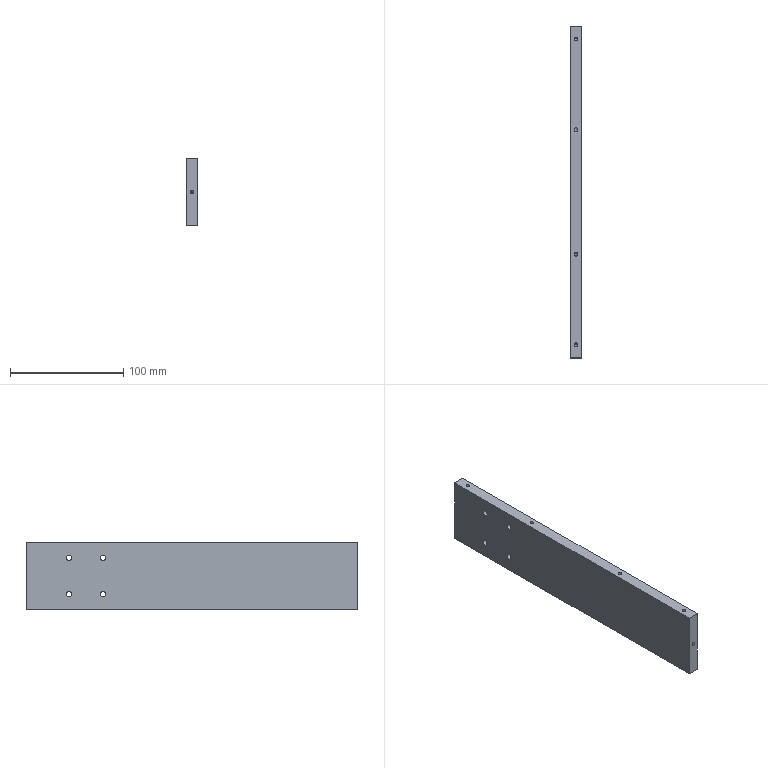Part | SolidWorks | features HoleWzd 3, MirrorPattern 2, Extrusion 1 | 1 solid | 54 faces | box 10 x 293 x 60 mm | volume 174003 mm3 | cylinder 28 | cone 20 | plane 6 | commonest cylinder face diameters 3.3 x20 5 x8
STEP:
#1=CARTESIAN_POINT('',(1.65,135.,-18.5));
#2=VERTEX_POINT('',#1);
#3=CARTESIAN_POINT('',(-1.65,135.,-18.5));
#4=VERTEX_POINT('',#3);
#5=CARTESIAN_POINT('',(0.,135.,-18.5));
#6=DIRECTION('',(0.,0.,-1.));
#7=DIRECTION('',(-1.,0.,0.));
#8=AXIS2_PLACEMENT_3D('',#5,#6,#7);
#9=CIRCLE('',#8,1.65);
#10=EDGE_CURVE('',#2,#4,#9,.T.);
#11=ORIENTED_EDGE('',*,*,#10,.F.);
#12=CARTESIAN_POINT('',(1.65,135.,-30.));
#13=VERTEX_POINT('',#12);
#14=CARTESIAN_POINT('',(1.65,135.,-30.));
#15=DIRECTION('',(0.,0.,-1.));
#16=VECTOR('',#15,1000.);
#17=LINE('',#14,#16);
#18=EDGE_CURVE('',#2,#13,#17,.T.);
#19=ORIENTED_EDGE('',*,*,#18,.T.);
#20=CARTESIAN_POINT('',(-1.65,135.,-30.));
#21=VERTEX_POINT('',#20);
#22=CARTESIAN_POINT('',(0.,135.,-30.));
#23=DIRECTION('',(0.,0.,-1.));
#24=DIRECTION('',(-1.,0.,0.));
#25=AXIS2_PLACEMENT_3D('',#22,#23,#24);
#26=CIRCLE('',#25,1.65);
#27=EDGE_CURVE('',#13,#21,#26,.T.);
#28=ORIENTED_EDGE('',*,*,#27,.T.);
#29=CARTESIAN_POINT('',(-1.65,135.,-30.));
#30=DIRECTION('',(0.,0.,-1.));
#31=VECTOR('',#30,1000.);
#32=LINE('',#29,#31);
#33=EDGE_CURVE('',#4,#21,#32,.T.);
#34=ORIENTED_EDGE('',*,*,#33,.F.);
#35=EDGE_LOOP('',(#11,#19,#28,#34));
#36=FACE_OUTER_BOUND('',#35,.T.);
#37=CARTESIAN_POINT('',(0.,135.,-30.));
#38=DIRECTION('',(0.,0.,-1.));
#39=DIRECTION('',(-1.,0.,0.));
#40=AXIS2_PLACEMENT_3D('',#37,#38,#39);
#41=CYLINDRICAL_SURFACE('',#40,1.65);
#42=ADVANCED_FACE('',(#36),#41,.F.);
#43=CARTESIAN_POINT('',(0.,135.,-17.509));
#44=VERTEX_POINT('',#43);
#45=CARTESIAN_POINT('',(-1.65,135.,-18.5));
#46=DIRECTION('',(-0.8572,0.,-0.515));
#47=VECTOR('',#46,1000.);
#48=LINE('',#45,#47);
#49=EDGE_CURVE('',#44,#4,#48,.T.);
#50=ORIENTED_EDGE('',*,*,#49,.F.);
#51=CARTESIAN_POINT('',(1.65,135.,-18.5));
#52=DIRECTION('',(0.8572,0.,-0.515));
#53=VECTOR('',#52,1000.);
#54=LINE('',#51,#53);
#55=EDGE_CURVE('',#44,#2,#54,.T.);
#56=ORIENTED_EDGE('',*,*,#55,.T.);
#57=ORIENTED_EDGE('',*,*,#10,.T.);
#58=EDGE_LOOP('',(#50,#56,#57));
#59=FACE_OUTER_BOUND('',#58,.T.);
#60=CARTESIAN_POINT('',(0.,135.,-18.5));
#61=DIRECTION('',(0.,0.,-1.));
#62=DIRECTION('',(-1.,0.,0.));
#63=AXIS2_PLACEMENT_3D('',#60,#61,#62);
#64=CONICAL_SURFACE('',#63,1.65,1.03);
#65=ADVANCED_FACE('',(#59),#64,.F.);
#66=CARTESIAN_POINT('',(1.65,-135.,-18.5));
#67=VERTEX_POINT('',#66);
#68=CARTESIAN_POINT('',(-1.65,-135.,-18.5));
#69=VERTEX_POINT('',#68);
#70=CARTESIAN_POINT('',(0.,-135.,-18.5));
#71=DIRECTION('',(0.,0.,-1.));
#72=DIRECTION('',(-1.,0.,0.));
#73=AXIS2_PLACEMENT_3D('',#70,#71,#72);
#74=CIRCLE('',#73,1.65);
#75=EDGE_CURVE('',#67,#69,#74,.T.);
#76=ORIENTED_EDGE('',*,*,#75,.F.);
#77=CARTESIAN_POINT('',(1.65,-135.,-30.));
#78=VERTEX_POINT('',#77);
#79=CARTESIAN_POINT('',(1.65,-135.,-30.));
#80=DIRECTION('',(0.,0.,-1.));
#81=VECTOR('',#80,1000.);
#82=LINE('',#79,#81);
#83=EDGE_CURVE('',#67,#78,#82,.T.);
#84=ORIENTED_EDGE('',*,*,#83,.T.);
#85=CARTESIAN_POINT('',(-1.65,-135.,-30.));
#86=VERTEX_POINT('',#85);
#87=CARTESIAN_POINT('',(0.,-135.,-30.));
#88=DIRECTION('',(0.,0.,-1.));
#89=DIRECTION('',(-1.,0.,0.));
#90=AXIS2_PLACEMENT_3D('',#87,#88,#89);
#91=CIRCLE('',#90,1.65);
#92=EDGE_CURVE('',#78,#86,#91,.T.);
#93=ORIENTED_EDGE('',*,*,#92,.T.);
#94=CARTESIAN_POINT('',(-1.65,-135.,-30.));
#95=DIRECTION('',(0.,0.,-1.));
#96=VECTOR('',#95,1000.);
#97=LINE('',#94,#96);
#98=EDGE_CURVE('',#69,#86,#97,.T.);
#99=ORIENTED_EDGE('',*,*,#98,.F.);
#100=EDGE_LOOP('',(#76,#84,#93,#99));
#101=FACE_OUTER_BOUND('',#100,.T.);
#102=CARTESIAN_POINT('',(0.,-135.,-30.));
#103=DIRECTION('',(0.,0.,-1.));
#104=DIRECTION('',(-1.,0.,0.));
#105=AXIS2_PLACEMENT_3D('',#102,#103,#104);
#106=CYLINDRICAL_SURFACE('',#105,1.65);
#107=ADVANCED_FACE('',(#101),#106,.F.);
#108=CARTESIAN_POINT('',(0.,-135.,-17.509));
#109=VERTEX_POINT('',#108);
#110=CARTESIAN_POINT('',(-1.65,-135.,-18.5));
#111=DIRECTION('',(-0.8572,0.,-0.515));
#112=VECTOR('',#111,1000.);
#113=LINE('',#110,#112);
#114=EDGE_CURVE('',#109,#69,#113,.T.);
#115=ORIENTED_EDGE('',*,*,#114,.F.);
#116=CARTESIAN_POINT('',(1.65,-135.,-18.5));
#117=DIRECTION('',(0.8572,0.,-0.515));
#118=VECTOR('',#117,1000.);
#119=LINE('',#116,#118);
#120=EDGE_CURVE('',#109,#67,#119,.T.);
#121=ORIENTED_EDGE('',*,*,#120,.T.);
#122=ORIENTED_EDGE('',*,*,#75,.T.);
#123=EDGE_LOOP('',(#115,#121,#122));
#124=FACE_OUTER_BOUND('',#123,.T.);
#125=CARTESIAN_POINT('',(0.,-135.,-18.5));
#126=DIRECTION('',(0.,0.,-1.));
#127=DIRECTION('',(-1.,0.,0.));
#128=AXIS2_PLACEMENT_3D('',#125,#126,#127);
#129=CONICAL_SURFACE('',#128,1.65,1.03);
#130=ADVANCED_FACE('',(#124),#129,.F.);
#131=CARTESIAN_POINT('',(1.65,55.,-18.5));
#132=VERTEX_POINT('',#131);
#133=CARTESIAN_POINT('',(-1.65,55.,-18.5));
#134=VERTEX_POINT('',#133);
#135=CARTESIAN_POINT('',(0.,55.,-18.5));
#136=DIRECTION('',(0.,0.,-1.));
#137=DIRECTION('',(-1.,0.,0.));
#138=AXIS2_PLACEMENT_3D('',#135,#136,#137);
#139=CIRCLE('',#138,1.65);
#140=EDGE_CURVE('',#132,#134,#139,.T.);
#141=ORIENTED_EDGE('',*,*,#140,.F.);
#142=CARTESIAN_POINT('',(1.65,55.,-30.));
#143=VERTEX_POINT('',#142);
#144=CARTESIAN_POINT('',(1.65,55.,-30.));
#145=DIRECTION('',(0.,0.,-1.));
#146=VECTOR('',#145,1000.);
#147=LINE('',#144,#146);
#148=EDGE_CURVE('',#132,#143,#147,.T.);
#149=ORIENTED_EDGE('',*,*,#148,.T.);
#150=CARTESIAN_POINT('',(-1.65,55.,-30.));
#151=VERTEX_POINT('',#150);
#152=CARTESIAN_POINT('',(0.,55.,-30.));
#153=DIRECTION('',(0.,0.,-1.));
#154=DIRECTION('',(-1.,0.,0.));
#155=AXIS2_PLACEMENT_3D('',#152,#153,#154);
#156=CIRCLE('',#155,1.65);
#157=EDGE_CURVE('',#143,#151,#156,.T.);
#158=ORIENTED_EDGE('',*,*,#157,.T.);
#159=CARTESIAN_POINT('',(-1.65,55.,-30.));
#160=DIRECTION('',(0.,0.,-1.));
#161=VECTOR('',#160,1000.);
#162=LINE('',#159,#161);
#163=EDGE_CURVE('',#134,#151,#162,.T.);
#164=ORIENTED_EDGE('',*,*,#163,.F.);
#165=EDGE_LOOP('',(#141,#149,#158,#164));
#166=FACE_OUTER_BOUND('',#165,.T.);
#167=CARTESIAN_POINT('',(0.,55.,-30.));
#168=DIRECTION('',(0.,0.,-1.));
#169=DIRECTION('',(-1.,0.,0.));
#170=AXIS2_PLACEMENT_3D('',#167,#168,#169);
#171=CYLINDRICAL_SURFACE('',#170,1.65);
#172=ADVANCED_FACE('',(#166),#171,.F.);
#173=CARTESIAN_POINT('',(0.,55.,-17.509));
#174=VERTEX_POINT('',#173);
#175=CARTESIAN_POINT('',(-1.65,55.,-18.5));
#176=DIRECTION('',(-0.8572,0.,-0.515));
#177=VECTOR('',#176,1000.);
#178=LINE('',#175,#177);
#179=EDGE_CURVE('',#174,#134,#178,.T.);
#180=ORIENTED_EDGE('',*,*,#179,.F.);
#181=CARTESIAN_POINT('',(1.65,55.,-18.5));
#182=DIRECTION('',(0.8572,0.,-0.515));
#183=VECTOR('',#182,1000.);
#184=LINE('',#181,#183);
#185=EDGE_CURVE('',#174,#132,#184,.T.);
#186=ORIENTED_EDGE('',*,*,#185,.T.);
#187=ORIENTED_EDGE('',*,*,#140,.T.);
#188=EDGE_LOOP('',(#180,#186,#187));
#189=FACE_OUTER_BOUND('',#188,.T.);
#190=CARTESIAN_POINT('',(0.,55.,-18.5));
#191=DIRECTION('',(0.,0.,-1.));
#192=DIRECTION('',(-1.,0.,0.));
#193=AXIS2_PLACEMENT_3D('',#190,#191,#192);
#194=CONICAL_SURFACE('',#193,1.65,1.03);
#195=ADVANCED_FACE('',(#189),#194,.F.);
#196=CARTESIAN_POINT('',(1.65,-55.,-18.5));
#197=VERTEX_POINT('',#196);
#198=CARTESIAN_POINT('',(-1.65,-55.,-18.5));
#199=VERTEX_POINT('',#198);
#200=CARTESIAN_POINT('',(0.,-55.,-18.5));
#201=DIRECTION('',(0.,0.,-1.));
#202=DIRECTION('',(-1.,0.,0.));
#203=AXIS2_PLACEMENT_3D('',#200,#201,#202);
#204=CIRCLE('',#203,1.65);
#205=EDGE_CURVE('',#197,#199,#204,.T.);
#206=ORIENTED_EDGE('',*,*,#205,.F.);
#207=CARTESIAN_POINT('',(1.65,-55.,-30.));
#208=VERTEX_POINT('',#207);
#209=CARTESIAN_POINT('',(1.65,-55.,-30.));
#210=DIRECTION('',(0.,0.,-1.));
#211=VECTOR('',#210,1000.);
#212=LINE('',#209,#211);
#213=EDGE_CURVE('',#197,#208,#212,.T.);
#214=ORIENTED_EDGE('',*,*,#213,.T.);
#215=CARTESIAN_POINT('',(-1.65,-55.,-30.));
#216=VERTEX_POINT('',#215);
#217=CARTESIAN_POINT('',(0.,-55.,-30.));
#218=DIRECTION('',(0.,0.,-1.));
#219=DIRECTION('',(-1.,0.,0.));
#220=AXIS2_PLACEMENT_3D('',#217,#218,#219);
#221=CIRCLE('',#220,1.65);
#222=EDGE_CURVE('',#208,#216,#221,.T.);
#223=ORIENTED_EDGE('',*,*,#222,.T.);
#224=CARTESIAN_POINT('',(-1.65,-55.,-30.));
#225=DIRECTION('',(0.,0.,-1.));
#226=VECTOR('',#225,1000.);
#227=LINE('',#224,#226);
#228=EDGE_CURVE('',#199,#216,#227,.T.);
#229=ORIENTED_EDGE('',*,*,#228,.F.);
#230=EDGE_LOOP('',(#206,#214,#223,#229));
#231=FACE_OUTER_BOUND('',#230,.T.);
#232=CARTESIAN_POINT('',(0.,-55.,-30.));
#233=DIRECTION('',(0.,0.,-1.));
#234=DIRECTION('',(-1.,0.,0.));
#235=AXIS2_PLACEMENT_3D('',#232,#233,#234);
#236=CYLINDRICAL_SURFACE('',#235,1.65);
#237=ADVANCED_FACE('',(#231),#236,.F.);
#238=CARTESIAN_POINT('',(0.,-55.,-17.509));
#239=VERTEX_POINT('',#238);
#240=CARTESIAN_POINT('',(-1.65,-55.,-18.5));
#241=DIRECTION('',(-0.8572,0.,-0.515));
#242=VECTOR('',#241,1000.);
#243=LINE('',#240,#242);
#244=EDGE_CURVE('',#239,#199,#243,.T.);
#245=ORIENTED_EDGE('',*,*,#244,.F.);
#246=CARTESIAN_POINT('',(1.65,-55.,-18.5));
#247=DIRECTION('',(0.8572,0.,-0.515));
#248=VECTOR('',#247,1000.);
#249=LINE('',#246,#248);
#250=EDGE_CURVE('',#239,#197,#249,.T.);
#251=ORIENTED_EDGE('',*,*,#250,.T.);
#252=ORIENTED_EDGE('',*,*,#205,.T.);
#253=EDGE_LOOP('',(#245,#251,#252));
#254=FACE_OUTER_BOUND('',#253,.T.);
#255=CARTESIAN_POINT('',(0.,-55.,-18.5));
#256=DIRECTION('',(0.,0.,-1.));
#257=DIRECTION('',(-1.,0.,0.));
#258=AXIS2_PLACEMENT_3D('',#255,#256,#257);
#259=CONICAL_SURFACE('',#258,1.65,1.03);
#260=ADVANCED_FACE('',(#254),#259,.F.);
#261=CARTESIAN_POINT('',(-5.,78.5,18.5));
#262=VERTEX_POINT('',#261);
#263=CARTESIAN_POINT('',(-5.,78.5,13.5));
#264=VERTEX_POINT('',#263);
#265=CARTESIAN_POINT('',(-5.,78.5,16.));
#266=DIRECTION('',(1.,0.,0.));
#267=DIRECTION('',(0.,0.,-1.));
#268=AXIS2_PLACEMENT_3D('',#265,#266,#267);
#269=CIRCLE('',#268,2.5);
#270=EDGE_CURVE('',#262,#264,#269,.T.);
#271=ORIENTED_EDGE('',*,*,#270,.F.);
#272=CARTESIAN_POINT('',(5.,78.5,18.5));
#273=VERTEX_POINT('',#272);
#274=CARTESIAN_POINT('',(5.,78.5,18.5));
#275=DIRECTION('',(1.,0.,0.));
#276=VECTOR('',#275,1000.);
#277=LINE('',#274,#276);
#278=EDGE_CURVE('',#262,#273,#277,.T.);
#279=ORIENTED_EDGE('',*,*,#278,.T.);
#280=CARTESIAN_POINT('',(5.,78.5,13.5));
#281=VERTEX_POINT('',#280);
#282=CARTESIAN_POINT('',(5.,78.5,16.));
#283=DIRECTION('',(1.,0.,0.));
#284=DIRECTION('',(0.,0.,-1.));
#285=AXIS2_PLACEMENT_3D('',#282,#283,#284);
#286=CIRCLE('',#285,2.5);
#287=EDGE_CURVE('',#273,#281,#286,.T.);
#288=ORIENTED_EDGE('',*,*,#287,.T.);
#289=CARTESIAN_POINT('',(5.,78.5,13.5));
#290=DIRECTION('',(1.,0.,0.));
#291=VECTOR('',#290,1000.);
#292=LINE('',#289,#291);
#293=EDGE_CURVE('',#264,#281,#292,.T.);
#294=ORIENTED_EDGE('',*,*,#293,.F.);
#295=EDGE_LOOP('',(#271,#279,#288,#294));
#296=FACE_OUTER_BOUND('',#295,.T.);
#297=CARTESIAN_POINT('',(5.,78.5,16.));
#298=DIRECTION('',(1.,0.,0.));
#299=DIRECTION('',(0.,0.,-1.));
#300=AXIS2_PLACEMENT_3D('',#297,#298,#299);
#301=CYLINDRICAL_SURFACE('',#300,2.5);
#302=ADVANCED_FACE('',(#296),#301,.F.);
#303=CARTESIAN_POINT('',(-5.,78.5,-13.5));
#304=VERTEX_POINT('',#303);
#305=CARTESIAN_POINT('',(-5.,78.5,-18.5));
#306=VERTEX_POINT('',#305);
#307=CARTESIAN_POINT('',(-5.,78.5,-16.));
#308=DIRECTION('',(1.,0.,0.));
#309=DIRECTION('',(0.,0.,-1.));
#310=AXIS2_PLACEMENT_3D('',#307,#308,#309);
#311=CIRCLE('',#310,2.5);
#312=EDGE_CURVE('',#304,#306,#311,.T.);
#313=ORIENTED_EDGE('',*,*,#312,.F.);
#314=CARTESIAN_POINT('',(5.,78.5,-13.5));
#315=VERTEX_POINT('',#314);
#316=CARTESIAN_POINT('',(5.,78.5,-13.5));
#317=DIRECTION('',(1.,0.,0.));
#318=VECTOR('',#317,1000.);
#319=LINE('',#316,#318);
#320=EDGE_CURVE('',#304,#315,#319,.T.);
#321=ORIENTED_EDGE('',*,*,#320,.T.);
#322=CARTESIAN_POINT('',(5.,78.5,-18.5));
#323=VERTEX_POINT('',#322);
#324=CARTESIAN_POINT('',(5.,78.5,-16.));
#325=DIRECTION('',(1.,0.,0.));
#326=DIRECTION('',(0.,0.,-1.));
#327=AXIS2_PLACEMENT_3D('',#324,#325,#326);
#328=CIRCLE('',#327,2.5);
#329=EDGE_CURVE('',#315,#323,#328,.T.);
#330=ORIENTED_EDGE('',*,*,#329,.T.);
#331=CARTESIAN_POINT('',(5.,78.5,-18.5));
#332=DIRECTION('',(1.,0.,0.));
#333=VECTOR('',#332,1000.);
#334=LINE('',#331,#333);
#335=EDGE_CURVE('',#306,#323,#334,.T.);
#336=ORIENTED_EDGE('',*,*,#335,.F.);
#337=EDGE_LOOP('',(#313,#321,#330,#336));
#338=FACE_OUTER_BOUND('',#337,.T.);
#339=CARTESIAN_POINT('',(5.,78.5,-16.));
#340=DIRECTION('',(1.,0.,0.));
#341=DIRECTION('',(0.,0.,-1.));
#342=AXIS2_PLACEMENT_3D('',#339,#340,#341);
#343=CYLINDRICAL_SURFACE('',#342,2.5);
#344=ADVANCED_FACE('',(#338),#343,.F.);
#345=CARTESIAN_POINT('',(-5.,108.5,-13.5));
#346=VERTEX_POINT('',#345);
#347=CARTESIAN_POINT('',(-5.,108.5,-18.5));
#348=VERTEX_POINT('',#347);
#349=CARTESIAN_POINT('',(-5.,108.5,-16.));
#350=DIRECTION('',(1.,0.,0.));
#351=DIRECTION('',(0.,0.,-1.));
#352=AXIS2_PLACEMENT_3D('',#349,#350,#351);
#353=CIRCLE('',#352,2.5);
#354=EDGE_CURVE('',#346,#348,#353,.T.);
#355=ORIENTED_EDGE('',*,*,#354,.F.);
#356=CARTESIAN_POINT('',(5.,108.5,-13.5));
#357=VERTEX_POINT('',#356);
#358=CARTESIAN_POINT('',(5.,108.5,-13.5));
#359=DIRECTION('',(1.,0.,0.));
#360=VECTOR('',#359,1000.);
#361=LINE('',#358,#360);
#362=EDGE_CURVE('',#346,#357,#361,.T.);
#363=ORIENTED_EDGE('',*,*,#362,.T.);
#364=CARTESIAN_POINT('',(5.,108.5,-18.5));
#365=VERTEX_POINT('',#364);
#366=CARTESIAN_POINT('',(5.,108.5,-16.));
#367=DIRECTION('',(1.,0.,0.));
#368=DIRECTION('',(0.,0.,-1.));
#369=AXIS2_PLACEMENT_3D('',#366,#367,#368);
#370=CIRCLE('',#369,2.5);
#371=EDGE_CURVE('',#357,#365,#370,.T.);
#372=ORIENTED_EDGE('',*,*,#371,.T.);
#373=CARTESIAN_POINT('',(5.,108.5,-18.5));
#374=DIRECTION('',(1.,0.,0.));
#375=VECTOR('',#374,1000.);
#376=LINE('',#373,#375);
#377=EDGE_CURVE('',#348,#365,#376,.T.);
#378=ORIENTED_EDGE('',*,*,#377,.F.);
#379=EDGE_LOOP('',(#355,#363,#372,#378));
#380=FACE_OUTER_BOUND('',#379,.T.);
#381=CARTESIAN_POINT('',(5.,108.5,-16.));
#382=DIRECTION('',(1.,0.,0.));
#383=DIRECTION('',(0.,0.,-1.));
#384=AXIS2_PLACEMENT_3D('',#381,#382,#383);
#385=CYLINDRICAL_SURFACE('',#384,2.5);
#386=ADVANCED_FACE('',(#380),#385,.F.);
#387=CARTESIAN_POINT('',(-5.,108.5,18.5));
#388=VERTEX_POINT('',#387);
#389=CARTESIAN_POINT('',(-5.,108.5,13.5));
#390=VERTEX_POINT('',#389);
#391=CARTESIAN_POINT('',(-5.,108.5,16.));
#392=DIRECTION('',(1.,0.,0.));
#393=DIRECTION('',(0.,0.,-1.));
#394=AXIS2_PLACEMENT_3D('',#391,#392,#393);
#395=CIRCLE('',#394,2.5);
#396=EDGE_CURVE('',#388,#390,#395,.T.);
#397=ORIENTED_EDGE('',*,*,#396,.F.);
#398=CARTESIAN_POINT('',(5.,108.5,18.5));
#399=VERTEX_POINT('',#398);
#400=CARTESIAN_POINT('',(5.,108.5,18.5));
#401=DIRECTION('',(1.,0.,0.));
#402=VECTOR('',#401,1000.);
#403=LINE('',#400,#402);
#404=EDGE_CURVE('',#388,#399,#403,.T.);
#405=ORIENTED_EDGE('',*,*,#404,.T.);
#406=CARTESIAN_POINT('',(5.,108.5,13.5));
#407=VERTEX_POINT('',#406);
#408=CARTESIAN_POINT('',(5.,108.5,16.));
#409=DIRECTION('',(1.,0.,0.));
#410=DIRECTION('',(0.,0.,-1.));
#411=AXIS2_PLACEMENT_3D('',#408,#409,#410);
#412=CIRCLE('',#411,2.5);
#413=EDGE_CURVE('',#399,#407,#412,.T.);
#414=ORIENTED_EDGE('',*,*,#413,.T.);
#415=CARTESIAN_POINT('',(5.,108.5,13.5));
#416=DIRECTION('',(1.,0.,0.));
#417=VECTOR('',#416,1000.);
#418=LINE('',#415,#417);
#419=EDGE_CURVE('',#390,#407,#418,.T.);
#420=ORIENTED_EDGE('',*,*,#419,.F.);
#421=EDGE_LOOP('',(#397,#405,#414,#420));
#422=FACE_OUTER_BOUND('',#421,.T.);
#423=CARTESIAN_POINT('',(5.,108.5,16.));
#424=DIRECTION('',(1.,0.,0.));
#425=DIRECTION('',(0.,0.,-1.));
#426=AXIS2_PLACEMENT_3D('',#423,#424,#425);
#427=CYLINDRICAL_SURFACE('',#426,2.5);
#428=ADVANCED_FACE('',(#422),#427,.F.);
#429=CARTESIAN_POINT('',(0.,135.,-1.65));
#430=VERTEX_POINT('',#429);
#431=CARTESIAN_POINT('',(0.,135.,1.65));
#432=VERTEX_POINT('',#431);
#433=CARTESIAN_POINT('',(0.,135.,0.));
#434=DIRECTION('',(0.,1.,0.));
#435=DIRECTION('',(0.,0.,1.));
#436=AXIS2_PLACEMENT_3D('',#433,#434,#435);
#437=CIRCLE('',#436,1.65);
#438=EDGE_CURVE('',#430,#432,#437,.T.);
#439=ORIENTED_EDGE('',*,*,#438,.F.);
#440=CARTESIAN_POINT('',(0.,146.5,-1.65));
#441=VERTEX_POINT('',#440);
#442=CARTESIAN_POINT('',(0.,146.5,-1.65));
#443=DIRECTION('',(0.,1.,0.));
#444=VECTOR('',#443,1000.);
#445=LINE('',#442,#444);
#446=EDGE_CURVE('',#430,#441,#445,.T.);
#447=ORIENTED_EDGE('',*,*,#446,.T.);
#448=CARTESIAN_POINT('',(0.,146.5,1.65));
#449=VERTEX_POINT('',#448);
#450=CARTESIAN_POINT('',(0.,146.5,0.));
#451=DIRECTION('',(0.,1.,0.));
#452=DIRECTION('',(0.,0.,1.));
#453=AXIS2_PLACEMENT_3D('',#450,#451,#452);
#454=CIRCLE('',#453,1.65);
#455=EDGE_CURVE('',#441,#449,#454,.T.);
#456=ORIENTED_EDGE('',*,*,#455,.T.);
#457=CARTESIAN_POINT('',(0.,146.5,1.65));
#458=DIRECTION('',(0.,1.,0.));
#459=VECTOR('',#458,1000.);
#460=LINE('',#457,#459);
#461=EDGE_CURVE('',#432,#449,#460,.T.);
#462=ORIENTED_EDGE('',*,*,#461,.F.);
#463=EDGE_LOOP('',(#439,#447,#456,#462));
#464=FACE_OUTER_BOUND('',#463,.T.);
#465=CARTESIAN_POINT('',(0.,146.5,0.));
#466=DIRECTION('',(0.,1.,0.));
#467=DIRECTION('',(0.,0.,1.));
#468=AXIS2_PLACEMENT_3D('',#465,#466,#467);
#469=CYLINDRICAL_SURFACE('',#468,1.65);
#470=ADVANCED_FACE('',(#464),#469,.F.);
#471=CARTESIAN_POINT('',(0.,134.009,0.));
#472=VERTEX_POINT('',#471);
#473=CARTESIAN_POINT('',(0.,135.,1.65));
#474=DIRECTION('',(0.,0.515,0.8572));
#475=VECTOR('',#474,1000.);
#476=LINE('',#473,#475);
#477=EDGE_CURVE('',#472,#432,#476,.T.);
#478=ORIENTED_EDGE('',*,*,#477,.F.);
#479=CARTESIAN_POINT('',(0.,135.,-1.65));
#480=DIRECTION('',(0.,0.515,-0.8572));
#481=VECTOR('',#480,1000.);
#482=LINE('',#479,#481);
#483=EDGE_CURVE('',#472,#430,#482,.T.);
#484=ORIENTED_EDGE('',*,*,#483,.T.);
#485=ORIENTED_EDGE('',*,*,#438,.T.);
#486=EDGE_LOOP('',(#478,#484,#485));
#487=FACE_OUTER_BOUND('',#486,.T.);
#488=CARTESIAN_POINT('',(0.,135.,0.));
#489=DIRECTION('',(0.,1.,0.));
#490=DIRECTION('',(0.,0.,1.));
#491=AXIS2_PLACEMENT_3D('',#488,#489,#490);
#492=CONICAL_SURFACE('',#491,1.65,1.03);
#493=ADVANCED_FACE('',(#487),#492,.F.);
#494=CARTESIAN_POINT('',(0.,-135.,1.65));
#495=VERTEX_POINT('',#494);
#496=CARTESIAN_POINT('',(0.,-135.,-1.65));
#497=VERTEX_POINT('',#496);
#498=CARTESIAN_POINT('',(0.,-135.,0.));
#499=DIRECTION('',(0.,-1.,0.));
#500=DIRECTION('',(0.,0.,-1.));
#501=AXIS2_PLACEMENT_3D('',#498,#499,#500);
#502=CIRCLE('',#501,1.65);
#503=EDGE_CURVE('',#495,#497,#502,.T.);
#504=ORIENTED_EDGE('',*,*,#503,.F.);
#505=CARTESIAN_POINT('',(0.,-146.5,1.65));
#506=VERTEX_POINT('',#505);
#507=CARTESIAN_POINT('',(0.,-146.5,1.65));
#508=DIRECTION('',(0.,-1.,0.));
#509=VECTOR('',#508,1000.);
#510=LINE('',#507,#509);
#511=EDGE_CURVE('',#495,#506,#510,.T.);
#512=ORIENTED_EDGE('',*,*,#511,.T.);
#513=CARTESIAN_POINT('',(0.,-146.5,-1.65));
#514=VERTEX_POINT('',#513);
#515=CARTESIAN_POINT('',(0.,-146.5,0.));
#516=DIRECTION('',(0.,-1.,0.));
#517=DIRECTION('',(0.,0.,-1.));
#518=AXIS2_PLACEMENT_3D('',#515,#516,#517);
#519=CIRCLE('',#518,1.65);
#520=EDGE_CURVE('',#506,#514,#519,.T.);
#521=ORIENTED_EDGE('',*,*,#520,.T.);
#522=CARTESIAN_POINT('',(0.,-146.5,-1.65));
#523=DIRECTION('',(0.,-1.,0.));
#524=VECTOR('',#523,1000.);
#525=LINE('',#522,#524);
#526=EDGE_CURVE('',#497,#514,#525,.T.);
#527=ORIENTED_EDGE('',*,*,#526,.F.);
#528=EDGE_LOOP('',(#504,#512,#521,#527));
#529=FACE_OUTER_BOUND('',#528,.T.);
#530=CARTESIAN_POINT('',(0.,-146.5,0.));
#531=DIRECTION('',(0.,-1.,0.));
#532=DIRECTION('',(0.,0.,-1.));
#533=AXIS2_PLACEMENT_3D('',#530,#531,#532);
#534=CYLINDRICAL_SURFACE('',#533,1.65);
#535=ADVANCED_FACE('',(#529),#534,.F.);
#536=CARTESIAN_POINT('',(0.,-134.009,0.));
#537=VERTEX_POINT('',#536);
#538=CARTESIAN_POINT('',(0.,-135.,-1.65));
#539=DIRECTION('',(0.,-0.515,-0.8572));
#540=VECTOR('',#539,1000.);
#541=LINE('',#538,#540);
#542=EDGE_CURVE('',#537,#497,#541,.T.);
#543=ORIENTED_EDGE('',*,*,#542,.F.);
#544=CARTESIAN_POINT('',(0.,-135.,1.65));
#545=DIRECTION('',(0.,-0.515,0.8572));
#546=VECTOR('',#545,1000.);
#547=LINE('',#544,#546);
#548=EDGE_CURVE('',#537,#495,#547,.T.);
#549=ORIENTED_EDGE('',*,*,#548,.T.);
#550=ORIENTED_EDGE('',*,*,#503,.T.);
#551=EDGE_LOOP('',(#543,#549,#550));
#552=FACE_OUTER_BOUND('',#551,.T.);
#553=CARTESIAN_POINT('',(0.,-135.,0.));
#554=DIRECTION('',(0.,-1.,0.));
#555=DIRECTION('',(0.,0.,-1.));
#556=AXIS2_PLACEMENT_3D('',#553,#554,#555);
#557=CONICAL_SURFACE('',#556,1.65,1.03);
#558=ADVANCED_FACE('',(#552),#557,.F.);
#559=CARTESIAN_POINT('',(-1.65,135.,18.5));
#560=VERTEX_POINT('',#559);
#561=CARTESIAN_POINT('',(1.65,135.,18.5));
#562=VERTEX_POINT('',#561);
#563=CARTESIAN_POINT('',(0.,135.,18.5));
#564=DIRECTION('',(0.,0.,1.));
#565=DIRECTION('',(1.,0.,0.));
#566=AXIS2_PLACEMENT_3D('',#563,#564,#565);
#567=CIRCLE('',#566,1.65);
#568=EDGE_CURVE('',#560,#562,#567,.T.);
#569=ORIENTED_EDGE('',*,*,#568,.F.);
#570=CARTESIAN_POINT('',(-1.65,135.,30.));
#571=VERTEX_POINT('',#570);
#572=CARTESIAN_POINT('',(-1.65,135.,30.));
#573=DIRECTION('',(0.,0.,1.));
#574=VECTOR('',#573,1000.);
#575=LINE('',#572,#574);
#576=EDGE_CURVE('',#560,#571,#575,.T.);
#577=ORIENTED_EDGE('',*,*,#576,.T.);
#578=CARTESIAN_POINT('',(1.65,135.,30.));
#579=VERTEX_POINT('',#578);
#580=CARTESIAN_POINT('',(0.,135.,30.));
#581=DIRECTION('',(0.,0.,1.));
#582=DIRECTION('',(1.,0.,0.));
#583=AXIS2_PLACEMENT_3D('',#580,#581,#582);
#584=CIRCLE('',#583,1.65);
#585=EDGE_CURVE('',#571,#579,#584,.T.);
#586=ORIENTED_EDGE('',*,*,#585,.T.);
#587=CARTESIAN_POINT('',(1.65,135.,30.));
#588=DIRECTION('',(0.,0.,1.));
#589=VECTOR('',#588,1000.);
#590=LINE('',#587,#589);
#591=EDGE_CURVE('',#562,#579,#590,.T.);
#592=ORIENTED_EDGE('',*,*,#591,.F.);
#593=EDGE_LOOP('',(#569,#577,#586,#592));
#594=FACE_OUTER_BOUND('',#593,.T.);
#595=CARTESIAN_POINT('',(0.,135.,30.));
#596=DIRECTION('',(0.,0.,1.));
#597=DIRECTION('',(1.,0.,0.));
#598=AXIS2_PLACEMENT_3D('',#595,#596,#597);
#599=CYLINDRICAL_SURFACE('',#598,1.65);
#600=ADVANCED_FACE('',(#594),#599,.F.);
#601=CARTESIAN_POINT('',(0.,135.,17.509));
#602=VERTEX_POINT('',#601);
#603=CARTESIAN_POINT('',(1.65,135.,18.5));
#604=DIRECTION('',(0.8572,0.,0.515));
#605=VECTOR('',#604,1000.);
#606=LINE('',#603,#605);
#607=EDGE_CURVE('',#602,#562,#606,.T.);
#608=ORIENTED_EDGE('',*,*,#607,.F.);
#609=CARTESIAN_POINT('',(-1.65,135.,18.5));
#610=DIRECTION('',(-0.8572,0.,0.515));
#611=VECTOR('',#610,1000.);
#612=LINE('',#609,#611);
#613=EDGE_CURVE('',#602,#560,#612,.T.);
#614=ORIENTED_EDGE('',*,*,#613,.T.);
#615=ORIENTED_EDGE('',*,*,#568,.T.);
#616=EDGE_LOOP('',(#608,#614,#615));
#617=FACE_OUTER_BOUND('',#616,.T.);
#618=CARTESIAN_POINT('',(0.,135.,18.5));
#619=DIRECTION('',(0.,0.,1.));
#620=DIRECTION('',(1.,0.,0.));
#621=AXIS2_PLACEMENT_3D('',#618,#619,#620);
#622=CONICAL_SURFACE('',#621,1.65,1.03);
#623=ADVANCED_FACE('',(#617),#622,.F.);
#624=CARTESIAN_POINT('',(-1.65,-135.,18.5));
#625=VERTEX_POINT('',#624);
#626=CARTESIAN_POINT('',(1.65,-135.,18.5));
#627=VERTEX_POINT('',#626);
#628=CARTESIAN_POINT('',(0.,-135.,18.5));
#629=DIRECTION('',(0.,0.,1.));
#630=DIRECTION('',(1.,0.,0.));
#631=AXIS2_PLACEMENT_3D('',#628,#629,#630);
#632=CIRCLE('',#631,1.65);
#633=EDGE_CURVE('',#625,#627,#632,.T.);
#634=ORIENTED_EDGE('',*,*,#633,.F.);
#635=CARTESIAN_POINT('',(-1.65,-135.,30.));
#636=VERTEX_POINT('',#635);
#637=CARTESIAN_POINT('',(-1.65,-135.,30.));
#638=DIRECTION('',(0.,0.,1.));
#639=VECTOR('',#638,1000.);
#640=LINE('',#637,#639);
#641=EDGE_CURVE('',#625,#636,#640,.T.);
#642=ORIENTED_EDGE('',*,*,#641,.T.);
#643=CARTESIAN_POINT('',(1.65,-135.,30.));
#644=VERTEX_POINT('',#643);
#645=CARTESIAN_POINT('',(0.,-135.,30.));
#646=DIRECTION('',(0.,0.,1.));
#647=DIRECTION('',(1.,0.,0.));
#648=AXIS2_PLACEMENT_3D('',#645,#646,#647);
#649=CIRCLE('',#648,1.65);
#650=EDGE_CURVE('',#636,#644,#649,.T.);
#651=ORIENTED_EDGE('',*,*,#650,.T.);
#652=CARTESIAN_POINT('',(1.65,-135.,30.));
#653=DIRECTION('',(0.,0.,1.));
#654=VECTOR('',#653,1000.);
#655=LINE('',#652,#654);
#656=EDGE_CURVE('',#627,#644,#655,.T.);
#657=ORIENTED_EDGE('',*,*,#656,.F.);
#658=EDGE_LOOP('',(#634,#642,#651,#657));
#659=FACE_OUTER_BOUND('',#658,.T.);
#660=CARTESIAN_POINT('',(0.,-135.,30.));
#661=DIRECTION('',(0.,0.,1.));
#662=DIRECTION('',(1.,0.,0.));
#663=AXIS2_PLACEMENT_3D('',#660,#661,#662);
#664=CYLINDRICAL_SURFACE('',#663,1.65);
#665=ADVANCED_FACE('',(#659),#664,.F.);
#666=CARTESIAN_POINT('',(0.,-135.,17.509));
#667=VERTEX_POINT('',#666);
#668=CARTESIAN_POINT('',(1.65,-135.,18.5));
#669=DIRECTION('',(0.8572,0.,0.515));
#670=VECTOR('',#669,1000.);
#671=LINE('',#668,#670);
#672=EDGE_CURVE('',#667,#627,#671,.T.);
#673=ORIENTED_EDGE('',*,*,#672,.F.);
#674=CARTESIAN_POINT('',(-1.65,-135.,18.5));
#675=DIRECTION('',(-0.8572,0.,0.515));
#676=VECTOR('',#675,1000.);
#677=LINE('',#674,#676);
#678=EDGE_CURVE('',#667,#625,#677,.T.);
#679=ORIENTED_EDGE('',*,*,#678,.T.);
#680=ORIENTED_EDGE('',*,*,#633,.T.);
#681=EDGE_LOOP('',(#673,#679,#680));
#682=FACE_OUTER_BOUND('',#681,.T.);
#683=CARTESIAN_POINT('',(0.,-135.,18.5));
#684=DIRECTION('',(0.,0.,1.));
#685=DIRECTION('',(1.,0.,0.));
#686=AXIS2_PLACEMENT_3D('',#683,#684,#685);
#687=CONICAL_SURFACE('',#686,1.65,1.03);
#688=ADVANCED_FACE('',(#682),#687,.F.);
#689=CARTESIAN_POINT('',(-1.65,55.,18.5));
#690=VERTEX_POINT('',#689);
#691=CARTESIAN_POINT('',(1.65,55.,18.5));
#692=VERTEX_POINT('',#691);
#693=CARTESIAN_POINT('',(0.,55.,18.5));
#694=DIRECTION('',(0.,0.,1.));
#695=DIRECTION('',(1.,0.,0.));
#696=AXIS2_PLACEMENT_3D('',#693,#694,#695);
#697=CIRCLE('',#696,1.65);
#698=EDGE_CURVE('',#690,#692,#697,.T.);
#699=ORIENTED_EDGE('',*,*,#698,.F.);
#700=CARTESIAN_POINT('',(-1.65,55.,30.));
#701=VERTEX_POINT('',#700);
#702=CARTESIAN_POINT('',(-1.65,55.,30.));
#703=DIRECTION('',(0.,0.,1.));
#704=VECTOR('',#703,1000.);
#705=LINE('',#702,#704);
#706=EDGE_CURVE('',#690,#701,#705,.T.);
#707=ORIENTED_EDGE('',*,*,#706,.T.);
#708=CARTESIAN_POINT('',(1.65,55.,30.));
#709=VERTEX_POINT('',#708);
#710=CARTESIAN_POINT('',(0.,55.,30.));
#711=DIRECTION('',(0.,0.,1.));
#712=DIRECTION('',(1.,0.,0.));
#713=AXIS2_PLACEMENT_3D('',#710,#711,#712);
#714=CIRCLE('',#713,1.65);
#715=EDGE_CURVE('',#701,#709,#714,.T.);
#716=ORIENTED_EDGE('',*,*,#715,.T.);
#717=CARTESIAN_POINT('',(1.65,55.,30.));
#718=DIRECTION('',(0.,0.,1.));
#719=VECTOR('',#718,1000.);
#720=LINE('',#717,#719);
#721=EDGE_CURVE('',#692,#709,#720,.T.);
#722=ORIENTED_EDGE('',*,*,#721,.F.);
#723=EDGE_LOOP('',(#699,#707,#716,#722));
#724=FACE_OUTER_BOUND('',#723,.T.);
#725=CARTESIAN_POINT('',(0.,55.,30.));
#726=DIRECTION('',(0.,0.,1.));
#727=DIRECTION('',(1.,0.,0.));
#728=AXIS2_PLACEMENT_3D('',#725,#726,#727);
#729=CYLINDRICAL_SURFACE('',#728,1.65);
#730=ADVANCED_FACE('',(#724),#729,.F.);
#731=CARTESIAN_POINT('',(0.,55.,17.509));
#732=VERTEX_POINT('',#731);
#733=CARTESIAN_POINT('',(1.65,55.,18.5));
#734=DIRECTION('',(0.8572,0.,0.515));
#735=VECTOR('',#734,1000.);
#736=LINE('',#733,#735);
#737=EDGE_CURVE('',#732,#692,#736,.T.);
#738=ORIENTED_EDGE('',*,*,#737,.F.);
#739=CARTESIAN_POINT('',(-1.65,55.,18.5));
#740=DIRECTION('',(-0.8572,0.,0.515));
#741=VECTOR('',#740,1000.);
#742=LINE('',#739,#741);
#743=EDGE_CURVE('',#732,#690,#742,.T.);
#744=ORIENTED_EDGE('',*,*,#743,.T.);
#745=ORIENTED_EDGE('',*,*,#698,.T.);
#746=EDGE_LOOP('',(#738,#744,#745));
#747=FACE_OUTER_BOUND('',#746,.T.);
#748=CARTESIAN_POINT('',(0.,55.,18.5));
#749=DIRECTION('',(0.,0.,1.));
#750=DIRECTION('',(1.,0.,0.));
#751=AXIS2_PLACEMENT_3D('',#748,#749,#750);
#752=CONICAL_SURFACE('',#751,1.65,1.03);
#753=ADVANCED_FACE('',(#747),#752,.F.);
#754=CARTESIAN_POINT('',(-1.65,-55.,18.5));
#755=VERTEX_POINT('',#754);
#756=CARTESIAN_POINT('',(1.65,-55.,18.5));
#757=VERTEX_POINT('',#756);
#758=CARTESIAN_POINT('',(0.,-55.,18.5));
#759=DIRECTION('',(0.,0.,1.));
#760=DIRECTION('',(1.,0.,0.));
#761=AXIS2_PLACEMENT_3D('',#758,#759,#760);
#762=CIRCLE('',#761,1.65);
#763=EDGE_CURVE('',#755,#757,#762,.T.);
#764=ORIENTED_EDGE('',*,*,#763,.F.);
#765=CARTESIAN_POINT('',(-1.65,-55.,30.));
#766=VERTEX_POINT('',#765);
#767=CARTESIAN_POINT('',(-1.65,-55.,30.));
#768=DIRECTION('',(0.,0.,1.));
#769=VECTOR('',#768,1000.);
#770=LINE('',#767,#769);
#771=EDGE_CURVE('',#755,#766,#770,.T.);
#772=ORIENTED_EDGE('',*,*,#771,.T.);
#773=CARTESIAN_POINT('',(1.65,-55.,30.));
#774=VERTEX_POINT('',#773);
#775=CARTESIAN_POINT('',(0.,-55.,30.));
#776=DIRECTION('',(0.,0.,1.));
#777=DIRECTION('',(1.,0.,0.));
#778=AXIS2_PLACEMENT_3D('',#775,#776,#777);
#779=CIRCLE('',#778,1.65);
#780=EDGE_CURVE('',#766,#774,#779,.T.);
#781=ORIENTED_EDGE('',*,*,#780,.T.);
#782=CARTESIAN_POINT('',(1.65,-55.,30.));
#783=DIRECTION('',(0.,0.,1.));
#784=VECTOR('',#783,1000.);
#785=LINE('',#782,#784);
#786=EDGE_CURVE('',#757,#774,#785,.T.);
#787=ORIENTED_EDGE('',*,*,#786,.F.);
#788=EDGE_LOOP('',(#764,#772,#781,#787));
#789=FACE_OUTER_BOUND('',#788,.T.);
#790=CARTESIAN_POINT('',(0.,-55.,30.));
#791=DIRECTION('',(0.,0.,1.));
#792=DIRECTION('',(1.,0.,0.));
#793=AXIS2_PLACEMENT_3D('',#790,#791,#792);
#794=CYLINDRICAL_SURFACE('',#793,1.65);
#795=ADVANCED_FACE('',(#789),#794,.F.);
#796=CARTESIAN_POINT('',(0.,-55.,17.509));
#797=VERTEX_POINT('',#796);
#798=CARTESIAN_POINT('',(1.65,-55.,18.5));
#799=DIRECTION('',(0.8572,0.,0.515));
#800=VECTOR('',#799,1000.);
#801=LINE('',#798,#800);
#802=EDGE_CURVE('',#797,#757,#801,.T.);
#803=ORIENTED_EDGE('',*,*,#802,.F.);
#804=CARTESIAN_POINT('',(-1.65,-55.,18.5));
#805=DIRECTION('',(-0.8572,0.,0.515));
#806=VECTOR('',#805,1000.);
#807=LINE('',#804,#806);
#808=EDGE_CURVE('',#797,#755,#807,.T.);
#809=ORIENTED_EDGE('',*,*,#808,.T.);
#810=ORIENTED_EDGE('',*,*,#763,.T.);
#811=EDGE_LOOP('',(#803,#809,#810));
#812=FACE_OUTER_BOUND('',#811,.T.);
#813=CARTESIAN_POINT('',(0.,-55.,18.5));
#814=DIRECTION('',(0.,0.,1.));
#815=DIRECTION('',(1.,0.,0.));
#816=AXIS2_PLACEMENT_3D('',#813,#814,#815);
#817=CONICAL_SURFACE('',#816,1.65,1.03);
#818=ADVANCED_FACE('',(#812),#817,.F.);
#819=CARTESIAN_POINT('',(-5.,78.5,16.));
#820=DIRECTION('',(1.,0.,0.));
#821=DIRECTION('',(0.,0.,-1.));
#822=AXIS2_PLACEMENT_3D('',#819,#820,#821);
#823=CIRCLE('',#822,2.5);
#824=EDGE_CURVE('',#264,#262,#823,.T.);
#825=ORIENTED_EDGE('',*,*,#824,.T.);
#826=ORIENTED_EDGE('',*,*,#270,.T.);
#827=EDGE_LOOP('',(#825,#826));
#828=FACE_BOUND('',#827,.T.);
#829=CARTESIAN_POINT('',(-5.,78.5,-16.));
#830=DIRECTION('',(1.,0.,0.));
#831=DIRECTION('',(0.,0.,-1.));
#832=AXIS2_PLACEMENT_3D('',#829,#830,#831);
#833=CIRCLE('',#832,2.5);
#834=EDGE_CURVE('',#306,#304,#833,.T.);
#835=ORIENTED_EDGE('',*,*,#834,.T.);
#836=ORIENTED_EDGE('',*,*,#312,.T.);
#837=EDGE_LOOP('',(#835,#836));
#838=FACE_BOUND('',#837,.T.);
#839=CARTESIAN_POINT('',(-5.,108.5,-16.));
#840=DIRECTION('',(1.,0.,0.));
#841=DIRECTION('',(0.,0.,-1.));
#842=AXIS2_PLACEMENT_3D('',#839,#840,#841);
#843=CIRCLE('',#842,2.5);
#844=EDGE_CURVE('',#348,#346,#843,.T.);
#845=ORIENTED_EDGE('',*,*,#844,.T.);
#846=ORIENTED_EDGE('',*,*,#354,.T.);
#847=EDGE_LOOP('',(#845,#846));
#848=FACE_BOUND('',#847,.T.);
#849=CARTESIAN_POINT('',(-5.,108.5,16.));
#850=DIRECTION('',(1.,0.,0.));
#851=DIRECTION('',(0.,0.,-1.));
#852=AXIS2_PLACEMENT_3D('',#849,#850,#851);
#853=CIRCLE('',#852,2.5);
#854=EDGE_CURVE('',#390,#388,#853,.T.);
#855=ORIENTED_EDGE('',*,*,#854,.T.);
#856=ORIENTED_EDGE('',*,*,#396,.T.);
#857=EDGE_LOOP('',(#855,#856));
#858=FACE_BOUND('',#857,.T.);
#859=CARTESIAN_POINT('',(-5.,146.5,-30.));
#860=VERTEX_POINT('',#859);
#861=CARTESIAN_POINT('',(-5.,-146.5,-30.));
#862=VERTEX_POINT('',#861);
#863=CARTESIAN_POINT('',(-5.,146.5,-30.));
#864=DIRECTION('',(0.,-1.,0.));
#865=VECTOR('',#864,1000.);
#866=LINE('',#863,#865);
#867=EDGE_CURVE('',#860,#862,#866,.T.);
#868=ORIENTED_EDGE('',*,*,#867,.T.);
#869=CARTESIAN_POINT('',(-5.,-146.5,30.));
#870=VERTEX_POINT('',#869);
#871=CARTESIAN_POINT('',(-5.,-146.5,30.));
#872=DIRECTION('',(0.,0.,-1.));
#873=VECTOR('',#872,1000.);
#874=LINE('',#871,#873);
#875=EDGE_CURVE('',#870,#862,#874,.T.);
#876=ORIENTED_EDGE('',*,*,#875,.F.);
#877=CARTESIAN_POINT('',(-5.,146.5,30.));
#878=VERTEX_POINT('',#877);
#879=CARTESIAN_POINT('',(-5.,146.5,30.));
#880=DIRECTION('',(0.,-1.,0.));
#881=VECTOR('',#880,1000.);
#882=LINE('',#879,#881);
#883=EDGE_CURVE('',#878,#870,#882,.T.);
#884=ORIENTED_EDGE('',*,*,#883,.F.);
#885=CARTESIAN_POINT('',(-5.,146.5,30.));
#886=DIRECTION('',(0.,0.,-1.));
#887=VECTOR('',#886,1000.);
#888=LINE('',#885,#887);
#889=EDGE_CURVE('',#878,#860,#888,.T.);
#890=ORIENTED_EDGE('',*,*,#889,.T.);
#891=EDGE_LOOP('',(#868,#876,#884,#890));
#892=FACE_OUTER_BOUND('',#891,.T.);
#893=CARTESIAN_POINT('',(-5.,146.5,30.));
#894=DIRECTION('',(1.,0.,0.));
#895=DIRECTION('',(0.,1.,0.));
#896=AXIS2_PLACEMENT_3D('',#893,#894,#895);
#897=PLANE('',#896);
#898=ADVANCED_FACE('',(#828,#838,#848,#858,#892),#897,.F.);
#899=CARTESIAN_POINT('',(0.,-146.5,0.));
#900=DIRECTION('',(0.,-1.,0.));
#901=DIRECTION('',(0.,0.,-1.));
#902=AXIS2_PLACEMENT_3D('',#899,#900,#901);
#903=CIRCLE('',#902,1.65);
#904=EDGE_CURVE('',#514,#506,#903,.T.);
#905=ORIENTED_EDGE('',*,*,#904,.F.);
#906=ORIENTED_EDGE('',*,*,#520,.F.);
#907=EDGE_LOOP('',(#905,#906));
#908=FACE_BOUND('',#907,.T.);
#909=CARTESIAN_POINT('',(5.,-146.5,-30.));
#910=VERTEX_POINT('',#909);
#911=CARTESIAN_POINT('',(5.,-146.5,-30.));
#912=DIRECTION('',(1.,0.,0.));
#913=VECTOR('',#912,1000.);
#914=LINE('',#911,#913);
#915=EDGE_CURVE('',#862,#910,#914,.T.);
#916=ORIENTED_EDGE('',*,*,#915,.T.);
#917=CARTESIAN_POINT('',(5.,-146.5,30.));
#918=VERTEX_POINT('',#917);
#919=CARTESIAN_POINT('',(5.,-146.5,30.));
#920=DIRECTION('',(0.,0.,-1.));
#921=VECTOR('',#920,1000.);
#922=LINE('',#919,#921);
#923=EDGE_CURVE('',#918,#910,#922,.T.);
#924=ORIENTED_EDGE('',*,*,#923,.F.);
#925=CARTESIAN_POINT('',(5.,-146.5,30.));
#926=DIRECTION('',(1.,0.,0.));
#927=VECTOR('',#926,1000.);
#928=LINE('',#925,#927);
#929=EDGE_CURVE('',#870,#918,#928,.T.);
#930=ORIENTED_EDGE('',*,*,#929,.F.);
#931=ORIENTED_EDGE('',*,*,#875,.T.);
#932=EDGE_LOOP('',(#916,#924,#930,#931));
#933=FACE_OUTER_BOUND('',#932,.T.);
#934=CARTESIAN_POINT('',(5.,-146.5,30.));
#935=DIRECTION('',(0.,1.,0.));
#936=DIRECTION('',(0.,0.,1.));
#937=AXIS2_PLACEMENT_3D('',#934,#935,#936);
#938=PLANE('',#937);
#939=ADVANCED_FACE('',(#908,#933),#938,.F.);
#940=CARTESIAN_POINT('',(5.,78.5,16.));
#941=DIRECTION('',(1.,0.,0.));
#942=DIRECTION('',(0.,0.,-1.));
#943=AXIS2_PLACEMENT_3D('',#940,#941,#942);
#944=CIRCLE('',#943,2.5);
#945=EDGE_CURVE('',#281,#273,#944,.T.);
#946=ORIENTED_EDGE('',*,*,#945,.F.);
#947=ORIENTED_EDGE('',*,*,#287,.F.);
#948=EDGE_LOOP('',(#946,#947));
#949=FACE_BOUND('',#948,.T.);
#950=CARTESIAN_POINT('',(5.,78.5,-16.));
#951=DIRECTION('',(1.,0.,0.));
#952=DIRECTION('',(0.,0.,-1.));
#953=AXIS2_PLACEMENT_3D('',#950,#951,#952);
#954=CIRCLE('',#953,2.5);
#955=EDGE_CURVE('',#323,#315,#954,.T.);
#956=ORIENTED_EDGE('',*,*,#955,.F.);
#957=ORIENTED_EDGE('',*,*,#329,.F.);
#958=EDGE_LOOP('',(#956,#957));
#959=FACE_BOUND('',#958,.T.);
#960=CARTESIAN_POINT('',(5.,108.5,-16.));
#961=DIRECTION('',(1.,0.,0.));
#962=DIRECTION('',(0.,0.,-1.));
#963=AXIS2_PLACEMENT_3D('',#960,#961,#962);
#964=CIRCLE('',#963,2.5);
#965=EDGE_CURVE('',#365,#357,#964,.T.);
#966=ORIENTED_EDGE('',*,*,#965,.F.);
#967=ORIENTED_EDGE('',*,*,#371,.F.);
#968=EDGE_LOOP('',(#966,#967));
#969=FACE_BOUND('',#968,.T.);
#970=CARTESIAN_POINT('',(5.,108.5,16.));
#971=DIRECTION('',(1.,0.,0.));
#972=DIRECTION('',(0.,0.,-1.));
#973=AXIS2_PLACEMENT_3D('',#970,#971,#972);
#974=CIRCLE('',#973,2.5);
#975=EDGE_CURVE('',#407,#399,#974,.T.);
#976=ORIENTED_EDGE('',*,*,#975,.F.);
#977=ORIENTED_EDGE('',*,*,#413,.F.);
#978=EDGE_LOOP('',(#976,#977));
#979=FACE_BOUND('',#978,.T.);
#980=CARTESIAN_POINT('',(5.,146.5,-30.));
#981=VERTEX_POINT('',#980);
#982=CARTESIAN_POINT('',(5.,146.5,-30.));
#983=DIRECTION('',(0.,1.,0.));
#984=VECTOR('',#983,1000.);
#985=LINE('',#982,#984);
#986=EDGE_CURVE('',#910,#981,#985,.T.);
#987=ORIENTED_EDGE('',*,*,#986,.T.);
#988=CARTESIAN_POINT('',(5.,146.5,30.));
#989=VERTEX_POINT('',#988);
#990=CARTESIAN_POINT('',(5.,146.5,30.));
#991=DIRECTION('',(0.,0.,-1.));
#992=VECTOR('',#991,1000.);
#993=LINE('',#990,#992);
#994=EDGE_CURVE('',#989,#981,#993,.T.);
#995=ORIENTED_EDGE('',*,*,#994,.F.);
#996=CARTESIAN_POINT('',(5.,146.5,30.));
#997=DIRECTION('',(0.,1.,0.));
#998=VECTOR('',#997,1000.);
#999=LINE('',#996,#998);
#1000=EDGE_CURVE('',#918,#989,#999,.T.);
#1001=ORIENTED_EDGE('',*,*,#1000,.F.);
#1002=ORIENTED_EDGE('',*,*,#923,.T.);
#1003=EDGE_LOOP('',(#987,#995,#1001,#1002));
#1004=FACE_OUTER_BOUND('',#1003,.T.);
#1005=CARTESIAN_POINT('',(5.,146.5,30.));
#1006=DIRECTION('',(-1.,0.,0.));
#1007=DIRECTION('',(0.,-1.,0.));
#1008=AXIS2_PLACEMENT_3D('',#1005,#1006,#1007);
#1009=PLANE('',#1008);
#1010=ADVANCED_FACE('',(#949,#959,#969,#979,#1004),#1009,.F.);
#1011=CARTESIAN_POINT('',(0.,146.5,0.));
#1012=DIRECTION('',(0.,1.,0.));
#1013=DIRECTION('',(0.,0.,1.));
#1014=AXIS2_PLACEMENT_3D('',#1011,#1012,#1013);
#1015=CIRCLE('',#1014,1.65);
#1016=EDGE_CURVE('',#449,#441,#1015,.T.);
#1017=ORIENTED_EDGE('',*,*,#1016,.F.);
#1018=ORIENTED_EDGE('',*,*,#455,.F.);
#1019=EDGE_LOOP('',(#1017,#1018));
#1020=FACE_BOUND('',#1019,.T.);
#1021=CARTESIAN_POINT('',(5.,146.5,-30.));
#1022=DIRECTION('',(-1.,0.,0.));
#1023=VECTOR('',#1022,1000.);
#1024=LINE('',#1021,#1023);
#1025=EDGE_CURVE('',#981,#860,#1024,.T.);
#1026=ORIENTED_EDGE('',*,*,#1025,.T.);
#1027=ORIENTED_EDGE('',*,*,#889,.F.);
#1028=CARTESIAN_POINT('',(5.,146.5,30.));
#1029=DIRECTION('',(-1.,0.,0.));
#1030=VECTOR('',#1029,1000.);
#1031=LINE('',#1028,#1030);
#1032=EDGE_CURVE('',#989,#878,#1031,.T.);
#1033=ORIENTED_EDGE('',*,*,#1032,.F.);
#1034=ORIENTED_EDGE('',*,*,#994,.T.);
#1035=EDGE_LOOP('',(#1026,#1027,#1033,#1034));
#1036=FACE_OUTER_BOUND('',#1035,.T.);
#1037=CARTESIAN_POINT('',(5.,146.5,30.));
#1038=DIRECTION('',(0.,-1.,0.));
#1039=DIRECTION('',(0.,0.,-1.));
#1040=AXIS2_PLACEMENT_3D('',#1037,#1038,#1039);
#1041=PLANE('',#1040);
#1042=ADVANCED_FACE('',(#1020,#1036),#1041,.F.);
#1043=CARTESIAN_POINT('',(0.,135.,30.));
#1044=DIRECTION('',(0.,0.,1.));
#1045=DIRECTION('',(1.,0.,0.));
#1046=AXIS2_PLACEMENT_3D('',#1043,#1044,#1045);
#1047=CIRCLE('',#1046,1.65);
#1048=EDGE_CURVE('',#579,#571,#1047,.T.);
#1049=ORIENTED_EDGE('',*,*,#1048,.F.);
#1050=ORIENTED_EDGE('',*,*,#585,.F.);
#1051=EDGE_LOOP('',(#1049,#1050));
#1052=FACE_BOUND('',#1051,.T.);
#1053=CARTESIAN_POINT('',(0.,-135.,30.));
#1054=DIRECTION('',(0.,0.,1.));
#1055=DIRECTION('',(1.,0.,0.));
#1056=AXIS2_PLACEMENT_3D('',#1053,#1054,#1055);
#1057=CIRCLE('',#1056,1.65);
#1058=EDGE_CURVE('',#644,#636,#1057,.T.);
#1059=ORIENTED_EDGE('',*,*,#1058,.F.);
#1060=ORIENTED_EDGE('',*,*,#650,.F.);
#1061=EDGE_LOOP('',(#1059,#1060));
#1062=FACE_BOUND('',#1061,.T.);
#1063=CARTESIAN_POINT('',(0.,55.,30.));
#1064=DIRECTION('',(0.,0.,1.));
#1065=DIRECTION('',(1.,0.,0.));
#1066=AXIS2_PLACEMENT_3D('',#1063,#1064,#1065);
#1067=CIRCLE('',#1066,1.65);
#1068=EDGE_CURVE('',#709,#701,#1067,.T.);
#1069=ORIENTED_EDGE('',*,*,#1068,.F.);
#1070=ORIENTED_EDGE('',*,*,#715,.F.);
#1071=EDGE_LOOP('',(#1069,#1070));
#1072=FACE_BOUND('',#1071,.T.);
#1073=CARTESIAN_POINT('',(0.,-55.,30.));
#1074=DIRECTION('',(0.,0.,1.));
#1075=DIRECTION('',(1.,0.,0.));
#1076=AXIS2_PLACEMENT_3D('',#1073,#1074,#1075);
#1077=CIRCLE('',#1076,1.65);
#1078=EDGE_CURVE('',#774,#766,#1077,.T.);
#1079=ORIENTED_EDGE('',*,*,#1078,.F.);
#1080=ORIENTED_EDGE('',*,*,#780,.F.);
#1081=EDGE_LOOP('',(#1079,#1080));
#1082=FACE_BOUND('',#1081,.T.);
#1083=ORIENTED_EDGE('',*,*,#883,.T.);
#1084=ORIENTED_EDGE('',*,*,#929,.T.);
#1085=ORIENTED_EDGE('',*,*,#1000,.T.);
#1086=ORIENTED_EDGE('',*,*,#1032,.T.);
#1087=EDGE_LOOP('',(#1083,#1084,#1085,#1086));
#1088=FACE_OUTER_BOUND('',#1087,.T.);
#1089=CARTESIAN_POINT('',(0.,0.,30.));
#1090=DIRECTION('',(0.,0.,-1.));
#1091=DIRECTION('',(-1.,0.,0.));
#1092=AXIS2_PLACEMENT_3D('',#1089,#1090,#1091);
#1093=PLANE('',#1092);
#1094=ADVANCED_FACE('',(#1052,#1062,#1072,#1082,#1088),#1093,.F.);
#1095=CARTESIAN_POINT('',(0.,135.,-30.));
#1096=DIRECTION('',(0.,0.,-1.));
#1097=DIRECTION('',(-1.,0.,0.));
#1098=AXIS2_PLACEMENT_3D('',#1095,#1096,#1097);
#1099=CIRCLE('',#1098,1.65);
#1100=EDGE_CURVE('',#21,#13,#1099,.T.);
#1101=ORIENTED_EDGE('',*,*,#1100,.F.);
#1102=ORIENTED_EDGE('',*,*,#27,.F.);
#1103=EDGE_LOOP('',(#1101,#1102));
#1104=FACE_BOUND('',#1103,.T.);
#1105=CARTESIAN_POINT('',(0.,-135.,-30.));
#1106=DIRECTION('',(0.,0.,-1.));
#1107=DIRECTION('',(-1.,0.,0.));
#1108=AXIS2_PLACEMENT_3D('',#1105,#1106,#1107);
#1109=CIRCLE('',#1108,1.65);
#1110=EDGE_CURVE('',#86,#78,#1109,.T.);
#1111=ORIENTED_EDGE('',*,*,#1110,.F.);
#1112=ORIENTED_EDGE('',*,*,#92,.F.);
#1113=EDGE_LOOP('',(#1111,#1112));
#1114=FACE_BOUND('',#1113,.T.);
#1115=CARTESIAN_POINT('',(0.,55.,-30.));
#1116=DIRECTION('',(0.,0.,-1.));
#1117=DIRECTION('',(-1.,0.,0.));
#1118=AXIS2_PLACEMENT_3D('',#1115,#1116,#1117);
#1119=CIRCLE('',#1118,1.65);
#1120=EDGE_CURVE('',#151,#143,#1119,.T.);
#1121=ORIENTED_EDGE('',*,*,#1120,.F.);
#1122=ORIENTED_EDGE('',*,*,#157,.F.);
#1123=EDGE_LOOP('',(#1121,#1122));
#1124=FACE_BOUND('',#1123,.T.);
#1125=CARTESIAN_POINT('',(0.,-55.,-30.));
#1126=DIRECTION('',(0.,0.,-1.));
#1127=DIRECTION('',(-1.,0.,0.));
#1128=AXIS2_PLACEMENT_3D('',#1125,#1126,#1127);
#1129=CIRCLE('',#1128,1.65);
#1130=EDGE_CURVE('',#216,#208,#1129,.T.);
#1131=ORIENTED_EDGE('',*,*,#1130,.F.);
#1132=ORIENTED_EDGE('',*,*,#222,.F.);
#1133=EDGE_LOOP('',(#1131,#1132));
#1134=FACE_BOUND('',#1133,.T.);
#1135=ORIENTED_EDGE('',*,*,#867,.F.);
#1136=ORIENTED_EDGE('',*,*,#1025,.F.);
#1137=ORIENTED_EDGE('',*,*,#986,.F.);
#1138=ORIENTED_EDGE('',*,*,#915,.F.);
#1139=EDGE_LOOP('',(#1135,#1136,#1137,#1138));
#1140=FACE_OUTER_BOUND('',#1139,.T.);
#1141=CARTESIAN_POINT('',(0.,0.,-30.));
#1142=DIRECTION('',(0.,0.,-1.));
#1143=DIRECTION('',(-1.,0.,0.));
#1144=AXIS2_PLACEMENT_3D('',#1141,#1142,#1143);
#1145=PLANE('',#1144);
#1146=ADVANCED_FACE('',(#1104,#1114,#1124,#1134,#1140),#1145,.T.);
#1147=ORIENTED_EDGE('',*,*,#808,.F.);
#1148=ORIENTED_EDGE('',*,*,#802,.T.);
#1149=CARTESIAN_POINT('',(0.,-55.,18.5));
#1150=DIRECTION('',(0.,0.,1.));
#1151=DIRECTION('',(1.,0.,0.));
#1152=AXIS2_PLACEMENT_3D('',#1149,#1150,#1151);
#1153=CIRCLE('',#1152,1.65);
#1154=EDGE_CURVE('',#757,#755,#1153,.T.);
#1155=ORIENTED_EDGE('',*,*,#1154,.T.);
#1156=EDGE_LOOP('',(#1147,#1148,#1155));
#1157=FACE_OUTER_BOUND('',#1156,.T.);
#1158=CARTESIAN_POINT('',(0.,-55.,18.5));
#1159=DIRECTION('',(0.,0.,1.));
#1160=DIRECTION('',(1.,0.,0.));
#1161=AXIS2_PLACEMENT_3D('',#1158,#1159,#1160);
#1162=CONICAL_SURFACE('',#1161,1.65,1.03);
#1163=ADVANCED_FACE('',(#1157),#1162,.F.);
#1164=ORIENTED_EDGE('',*,*,#771,.F.);
#1165=ORIENTED_EDGE('',*,*,#1154,.F.);
#1166=ORIENTED_EDGE('',*,*,#786,.T.);
#1167=ORIENTED_EDGE('',*,*,#1078,.T.);
#1168=EDGE_LOOP('',(#1164,#1165,#1166,#1167));
#1169=FACE_OUTER_BOUND('',#1168,.T.);
#1170=CARTESIAN_POINT('',(0.,-55.,30.));
#1171=DIRECTION('',(0.,0.,1.));
#1172=DIRECTION('',(1.,0.,0.));
#1173=AXIS2_PLACEMENT_3D('',#1170,#1171,#1172);
#1174=CYLINDRICAL_SURFACE('',#1173,1.65);
#1175=ADVANCED_FACE('',(#1169),#1174,.F.);
#1176=ORIENTED_EDGE('',*,*,#743,.F.);
#1177=ORIENTED_EDGE('',*,*,#737,.T.);
#1178=CARTESIAN_POINT('',(0.,55.,18.5));
#1179=DIRECTION('',(0.,0.,1.));
#1180=DIRECTION('',(1.,0.,0.));
#1181=AXIS2_PLACEMENT_3D('',#1178,#1179,#1180);
#1182=CIRCLE('',#1181,1.65);
#1183=EDGE_CURVE('',#692,#690,#1182,.T.);
#1184=ORIENTED_EDGE('',*,*,#1183,.T.);
#1185=EDGE_LOOP('',(#1176,#1177,#1184));
#1186=FACE_OUTER_BOUND('',#1185,.T.);
#1187=CARTESIAN_POINT('',(0.,55.,18.5));
#1188=DIRECTION('',(0.,0.,1.));
#1189=DIRECTION('',(1.,0.,0.));
#1190=AXIS2_PLACEMENT_3D('',#1187,#1188,#1189);
#1191=CONICAL_SURFACE('',#1190,1.65,1.03);
#1192=ADVANCED_FACE('',(#1186),#1191,.F.);
#1193=ORIENTED_EDGE('',*,*,#706,.F.);
#1194=ORIENTED_EDGE('',*,*,#1183,.F.);
#1195=ORIENTED_EDGE('',*,*,#721,.T.);
#1196=ORIENTED_EDGE('',*,*,#1068,.T.);
#1197=EDGE_LOOP('',(#1193,#1194,#1195,#1196));
#1198=FACE_OUTER_BOUND('',#1197,.T.);
#1199=CARTESIAN_POINT('',(0.,55.,30.));
#1200=DIRECTION('',(0.,0.,1.));
#1201=DIRECTION('',(1.,0.,0.));
#1202=AXIS2_PLACEMENT_3D('',#1199,#1200,#1201);
#1203=CYLINDRICAL_SURFACE('',#1202,1.65);
#1204=ADVANCED_FACE('',(#1198),#1203,.F.);
#1205=ORIENTED_EDGE('',*,*,#678,.F.);
#1206=ORIENTED_EDGE('',*,*,#672,.T.);
#1207=CARTESIAN_POINT('',(0.,-135.,18.5));
#1208=DIRECTION('',(0.,0.,1.));
#1209=DIRECTION('',(1.,0.,0.));
#1210=AXIS2_PLACEMENT_3D('',#1207,#1208,#1209);
#1211=CIRCLE('',#1210,1.65);
#1212=EDGE_CURVE('',#627,#625,#1211,.T.);
#1213=ORIENTED_EDGE('',*,*,#1212,.T.);
#1214=EDGE_LOOP('',(#1205,#1206,#1213));
#1215=FACE_OUTER_BOUND('',#1214,.T.);
#1216=CARTESIAN_POINT('',(0.,-135.,18.5));
#1217=DIRECTION('',(0.,0.,1.));
#1218=DIRECTION('',(1.,0.,0.));
#1219=AXIS2_PLACEMENT_3D('',#1216,#1217,#1218);
#1220=CONICAL_SURFACE('',#1219,1.65,1.03);
#1221=ADVANCED_FACE('',(#1215),#1220,.F.);
#1222=ORIENTED_EDGE('',*,*,#641,.F.);
#1223=ORIENTED_EDGE('',*,*,#1212,.F.);
#1224=ORIENTED_EDGE('',*,*,#656,.T.);
#1225=ORIENTED_EDGE('',*,*,#1058,.T.);
#1226=EDGE_LOOP('',(#1222,#1223,#1224,#1225));
#1227=FACE_OUTER_BOUND('',#1226,.T.);
#1228=CARTESIAN_POINT('',(0.,-135.,30.));
#1229=DIRECTION('',(0.,0.,1.));
#1230=DIRECTION('',(1.,0.,0.));
#1231=AXIS2_PLACEMENT_3D('',#1228,#1229,#1230);
#1232=CYLINDRICAL_SURFACE('',#1231,1.65);
#1233=ADVANCED_FACE('',(#1227),#1232,.F.);
#1234=ORIENTED_EDGE('',*,*,#613,.F.);
#1235=ORIENTED_EDGE('',*,*,#607,.T.);
#1236=CARTESIAN_POINT('',(0.,135.,18.5));
#1237=DIRECTION('',(0.,0.,1.));
#1238=DIRECTION('',(1.,0.,0.));
#1239=AXIS2_PLACEMENT_3D('',#1236,#1237,#1238);
#1240=CIRCLE('',#1239,1.65);
#1241=EDGE_CURVE('',#562,#560,#1240,.T.);
#1242=ORIENTED_EDGE('',*,*,#1241,.T.);
#1243=EDGE_LOOP('',(#1234,#1235,#1242));
#1244=FACE_OUTER_BOUND('',#1243,.T.);
#1245=CARTESIAN_POINT('',(0.,135.,18.5));
#1246=DIRECTION('',(0.,0.,1.));
#1247=DIRECTION('',(1.,0.,0.));
#1248=AXIS2_PLACEMENT_3D('',#1245,#1246,#1247);
#1249=CONICAL_SURFACE('',#1248,1.65,1.03);
#1250=ADVANCED_FACE('',(#1244),#1249,.F.);
#1251=ORIENTED_EDGE('',*,*,#576,.F.);
#1252=ORIENTED_EDGE('',*,*,#1241,.F.);
#1253=ORIENTED_EDGE('',*,*,#591,.T.);
#1254=ORIENTED_EDGE('',*,*,#1048,.T.);
#1255=EDGE_LOOP('',(#1251,#1252,#1253,#1254));
#1256=FACE_OUTER_BOUND('',#1255,.T.);
#1257=CARTESIAN_POINT('',(0.,135.,30.));
#1258=DIRECTION('',(0.,0.,1.));
#1259=DIRECTION('',(1.,0.,0.));
#1260=AXIS2_PLACEMENT_3D('',#1257,#1258,#1259);
#1261=CYLINDRICAL_SURFACE('',#1260,1.65);
#1262=ADVANCED_FACE('',(#1256),#1261,.F.);
#1263=ORIENTED_EDGE('',*,*,#548,.F.);
#1264=ORIENTED_EDGE('',*,*,#542,.T.);
#1265=CARTESIAN_POINT('',(0.,-135.,0.));
#1266=DIRECTION('',(0.,-1.,0.));
#1267=DIRECTION('',(0.,0.,-1.));
#1268=AXIS2_PLACEMENT_3D('',#1265,#1266,#1267);
#1269=CIRCLE('',#1268,1.65);
#1270=EDGE_CURVE('',#497,#495,#1269,.T.);
#1271=ORIENTED_EDGE('',*,*,#1270,.T.);
#1272=EDGE_LOOP('',(#1263,#1264,#1271));
#1273=FACE_OUTER_BOUND('',#1272,.T.);
#1274=CARTESIAN_POINT('',(0.,-135.,0.));
#1275=DIRECTION('',(0.,-1.,0.));
#1276=DIRECTION('',(0.,0.,-1.));
#1277=AXIS2_PLACEMENT_3D('',#1274,#1275,#1276);
#1278=CONICAL_SURFACE('',#1277,1.65,1.03);
#1279=ADVANCED_FACE('',(#1273),#1278,.F.);
#1280=ORIENTED_EDGE('',*,*,#511,.F.);
#1281=ORIENTED_EDGE('',*,*,#1270,.F.);
#1282=ORIENTED_EDGE('',*,*,#526,.T.);
#1283=ORIENTED_EDGE('',*,*,#904,.T.);
#1284=EDGE_LOOP('',(#1280,#1281,#1282,#1283));
#1285=FACE_OUTER_BOUND('',#1284,.T.);
#1286=CARTESIAN_POINT('',(0.,-146.5,0.));
#1287=DIRECTION('',(0.,-1.,0.));
#1288=DIRECTION('',(0.,0.,-1.));
#1289=AXIS2_PLACEMENT_3D('',#1286,#1287,#1288);
#1290=CYLINDRICAL_SURFACE('',#1289,1.65);
#1291=ADVANCED_FACE('',(#1285),#1290,.F.);
#1292=ORIENTED_EDGE('',*,*,#483,.F.);
#1293=ORIENTED_EDGE('',*,*,#477,.T.);
#1294=CARTESIAN_POINT('',(0.,135.,0.));
#1295=DIRECTION('',(0.,1.,0.));
#1296=DIRECTION('',(0.,0.,1.));
#1297=AXIS2_PLACEMENT_3D('',#1294,#1295,#1296);
#1298=CIRCLE('',#1297,1.65);
#1299=EDGE_CURVE('',#432,#430,#1298,.T.);
#1300=ORIENTED_EDGE('',*,*,#1299,.T.);
#1301=EDGE_LOOP('',(#1292,#1293,#1300));
#1302=FACE_OUTER_BOUND('',#1301,.T.);
#1303=CARTESIAN_POINT('',(0.,135.,0.));
#1304=DIRECTION('',(0.,1.,0.));
#1305=DIRECTION('',(0.,0.,1.));
#1306=AXIS2_PLACEMENT_3D('',#1303,#1304,#1305);
#1307=CONICAL_SURFACE('',#1306,1.65,1.03);
#1308=ADVANCED_FACE('',(#1302),#1307,.F.);
#1309=ORIENTED_EDGE('',*,*,#446,.F.);
#1310=ORIENTED_EDGE('',*,*,#1299,.F.);
#1311=ORIENTED_EDGE('',*,*,#461,.T.);
#1312=ORIENTED_EDGE('',*,*,#1016,.T.);
#1313=EDGE_LOOP('',(#1309,#1310,#1311,#1312));
#1314=FACE_OUTER_BOUND('',#1313,.T.);
#1315=CARTESIAN_POINT('',(0.,146.5,0.));
#1316=DIRECTION('',(0.,1.,0.));
#1317=DIRECTION('',(0.,0.,1.));
#1318=AXIS2_PLACEMENT_3D('',#1315,#1316,#1317);
#1319=CYLINDRICAL_SURFACE('',#1318,1.65);
#1320=ADVANCED_FACE('',(#1314),#1319,.F.);
#1321=ORIENTED_EDGE('',*,*,#404,.F.);
#1322=ORIENTED_EDGE('',*,*,#854,.F.);
#1323=ORIENTED_EDGE('',*,*,#419,.T.);
#1324=ORIENTED_EDGE('',*,*,#975,.T.);
#1325=EDGE_LOOP('',(#1321,#1322,#1323,#1324));
#1326=FACE_OUTER_BOUND('',#1325,.T.);
#1327=CARTESIAN_POINT('',(5.,108.5,16.));
#1328=DIRECTION('',(1.,0.,0.));
#1329=DIRECTION('',(0.,0.,-1.));
#1330=AXIS2_PLACEMENT_3D('',#1327,#1328,#1329);
#1331=CYLINDRICAL_SURFACE('',#1330,2.5);
#1332=ADVANCED_FACE('',(#1326),#1331,.F.);
#1333=ORIENTED_EDGE('',*,*,#362,.F.);
#1334=ORIENTED_EDGE('',*,*,#844,.F.);
#1335=ORIENTED_EDGE('',*,*,#377,.T.);
#1336=ORIENTED_EDGE('',*,*,#965,.T.);
#1337=EDGE_LOOP('',(#1333,#1334,#1335,#1336));
#1338=FACE_OUTER_BOUND('',#1337,.T.);
#1339=CARTESIAN_POINT('',(5.,108.5,-16.));
#1340=DIRECTION('',(1.,0.,0.));
#1341=DIRECTION('',(0.,0.,-1.));
#1342=AXIS2_PLACEMENT_3D('',#1339,#1340,#1341);
#1343=CYLINDRICAL_SURFACE('',#1342,2.5);
#1344=ADVANCED_FACE('',(#1338),#1343,.F.);
#1345=ORIENTED_EDGE('',*,*,#320,.F.);
#1346=ORIENTED_EDGE('',*,*,#834,.F.);
#1347=ORIENTED_EDGE('',*,*,#335,.T.);
#1348=ORIENTED_EDGE('',*,*,#955,.T.);
#1349=EDGE_LOOP('',(#1345,#1346,#1347,#1348));
#1350=FACE_OUTER_BOUND('',#1349,.T.);
#1351=CARTESIAN_POINT('',(5.,78.5,-16.));
#1352=DIRECTION('',(1.,0.,0.));
#1353=DIRECTION('',(0.,0.,-1.));
#1354=AXIS2_PLACEMENT_3D('',#1351,#1352,#1353);
#1355=CYLINDRICAL_SURFACE('',#1354,2.5);
#1356=ADVANCED_FACE('',(#1350),#1355,.F.);
#1357=ORIENTED_EDGE('',*,*,#278,.F.);
#1358=ORIENTED_EDGE('',*,*,#824,.F.);
#1359=ORIENTED_EDGE('',*,*,#293,.T.);
#1360=ORIENTED_EDGE('',*,*,#945,.T.);
#1361=EDGE_LOOP('',(#1357,#1358,#1359,#1360));
#1362=FACE_OUTER_BOUND('',#1361,.T.);
#1363=CARTESIAN_POINT('',(5.,78.5,16.));
#1364=DIRECTION('',(1.,0.,0.));
#1365=DIRECTION('',(0.,0.,-1.));
#1366=AXIS2_PLACEMENT_3D('',#1363,#1364,#1365);
#1367=CYLINDRICAL_SURFACE('',#1366,2.5);
#1368=ADVANCED_FACE('',(#1362),#1367,.F.);
#1369=ORIENTED_EDGE('',*,*,#250,.F.);
#1370=ORIENTED_EDGE('',*,*,#244,.T.);
#1371=CARTESIAN_POINT('',(0.,-55.,-18.5));
#1372=DIRECTION('',(0.,0.,-1.));
#1373=DIRECTION('',(-1.,0.,0.));
#1374=AXIS2_PLACEMENT_3D('',#1371,#1372,#1373);
#1375=CIRCLE('',#1374,1.65);
#1376=EDGE_CURVE('',#199,#197,#1375,.T.);
#1377=ORIENTED_EDGE('',*,*,#1376,.T.);
#1378=EDGE_LOOP('',(#1369,#1370,#1377));
#1379=FACE_OUTER_BOUND('',#1378,.T.);
#1380=CARTESIAN_POINT('',(0.,-55.,-18.5));
#1381=DIRECTION('',(0.,0.,-1.));
#1382=DIRECTION('',(-1.,0.,0.));
#1383=AXIS2_PLACEMENT_3D('',#1380,#1381,#1382);
#1384=CONICAL_SURFACE('',#1383,1.65,1.03);
#1385=ADVANCED_FACE('',(#1379),#1384,.F.);
#1386=ORIENTED_EDGE('',*,*,#213,.F.);
#1387=ORIENTED_EDGE('',*,*,#1376,.F.);
#1388=ORIENTED_EDGE('',*,*,#228,.T.);
#1389=ORIENTED_EDGE('',*,*,#1130,.T.);
#1390=EDGE_LOOP('',(#1386,#1387,#1388,#1389));
#1391=FACE_OUTER_BOUND('',#1390,.T.);
#1392=CARTESIAN_POINT('',(0.,-55.,-30.));
#1393=DIRECTION('',(0.,0.,-1.));
#1394=DIRECTION('',(-1.,0.,0.));
#1395=AXIS2_PLACEMENT_3D('',#1392,#1393,#1394);
#1396=CYLINDRICAL_SURFACE('',#1395,1.65);
#1397=ADVANCED_FACE('',(#1391),#1396,.F.);
#1398=ORIENTED_EDGE('',*,*,#185,.F.);
#1399=ORIENTED_EDGE('',*,*,#179,.T.);
#1400=CARTESIAN_POINT('',(0.,55.,-18.5));
#1401=DIRECTION('',(0.,0.,-1.));
#1402=DIRECTION('',(-1.,0.,0.));
#1403=AXIS2_PLACEMENT_3D('',#1400,#1401,#1402);
#1404=CIRCLE('',#1403,1.65);
#1405=EDGE_CURVE('',#134,#132,#1404,.T.);
#1406=ORIENTED_EDGE('',*,*,#1405,.T.);
#1407=EDGE_LOOP('',(#1398,#1399,#1406));
#1408=FACE_OUTER_BOUND('',#1407,.T.);
#1409=CARTESIAN_POINT('',(0.,55.,-18.5));
#1410=DIRECTION('',(0.,0.,-1.));
#1411=DIRECTION('',(-1.,0.,0.));
#1412=AXIS2_PLACEMENT_3D('',#1409,#1410,#1411);
#1413=CONICAL_SURFACE('',#1412,1.65,1.03);
#1414=ADVANCED_FACE('',(#1408),#1413,.F.);
#1415=ORIENTED_EDGE('',*,*,#148,.F.);
#1416=ORIENTED_EDGE('',*,*,#1405,.F.);
#1417=ORIENTED_EDGE('',*,*,#163,.T.);
#1418=ORIENTED_EDGE('',*,*,#1120,.T.);
#1419=EDGE_LOOP('',(#1415,#1416,#1417,#1418));
#1420=FACE_OUTER_BOUND('',#1419,.T.);
#1421=CARTESIAN_POINT('',(0.,55.,-30.));
#1422=DIRECTION('',(0.,0.,-1.));
#1423=DIRECTION('',(-1.,0.,0.));
#1424=AXIS2_PLACEMENT_3D('',#1421,#1422,#1423);
#1425=CYLINDRICAL_SURFACE('',#1424,1.65);
#1426=ADVANCED_FACE('',(#1420),#1425,.F.);
#1427=ORIENTED_EDGE('',*,*,#120,.F.);
#1428=ORIENTED_EDGE('',*,*,#114,.T.);
#1429=CARTESIAN_POINT('',(0.,-135.,-18.5));
#1430=DIRECTION('',(0.,0.,-1.));
#1431=DIRECTION('',(-1.,0.,0.));
#1432=AXIS2_PLACEMENT_3D('',#1429,#1430,#1431);
#1433=CIRCLE('',#1432,1.65);
#1434=EDGE_CURVE('',#69,#67,#1433,.T.);
#1435=ORIENTED_EDGE('',*,*,#1434,.T.);
#1436=EDGE_LOOP('',(#1427,#1428,#1435));
#1437=FACE_OUTER_BOUND('',#1436,.T.);
#1438=CARTESIAN_POINT('',(0.,-135.,-18.5));
#1439=DIRECTION('',(0.,0.,-1.));
#1440=DIRECTION('',(-1.,0.,0.));
#1441=AXIS2_PLACEMENT_3D('',#1438,#1439,#1440);
#1442=CONICAL_SURFACE('',#1441,1.65,1.03);
#1443=ADVANCED_FACE('',(#1437),#1442,.F.);
#1444=ORIENTED_EDGE('',*,*,#83,.F.);
#1445=ORIENTED_EDGE('',*,*,#1434,.F.);
#1446=ORIENTED_EDGE('',*,*,#98,.T.);
#1447=ORIENTED_EDGE('',*,*,#1110,.T.);
#1448=EDGE_LOOP('',(#1444,#1445,#1446,#1447));
#1449=FACE_OUTER_BOUND('',#1448,.T.);
#1450=CARTESIAN_POINT('',(0.,-135.,-30.));
#1451=DIRECTION('',(0.,0.,-1.));
#1452=DIRECTION('',(-1.,0.,0.));
#1453=AXIS2_PLACEMENT_3D('',#1450,#1451,#1452);
#1454=CYLINDRICAL_SURFACE('',#1453,1.65);
#1455=ADVANCED_FACE('',(#1449),#1454,.F.);
#1456=ORIENTED_EDGE('',*,*,#55,.F.);
#1457=ORIENTED_EDGE('',*,*,#49,.T.);
#1458=CARTESIAN_POINT('',(0.,135.,-18.5));
#1459=DIRECTION('',(0.,0.,-1.));
#1460=DIRECTION('',(-1.,0.,0.));
#1461=AXIS2_PLACEMENT_3D('',#1458,#1459,#1460);
#1462=CIRCLE('',#1461,1.65);
#1463=EDGE_CURVE('',#4,#2,#1462,.T.);
#1464=ORIENTED_EDGE('',*,*,#1463,.T.);
#1465=EDGE_LOOP('',(#1456,#1457,#1464));
#1466=FACE_OUTER_BOUND('',#1465,.T.);
#1467=CARTESIAN_POINT('',(0.,135.,-18.5));
#1468=DIRECTION('',(0.,0.,-1.));
#1469=DIRECTION('',(-1.,0.,0.));
#1470=AXIS2_PLACEMENT_3D('',#1467,#1468,#1469);
#1471=CONICAL_SURFACE('',#1470,1.65,1.03);
#1472=ADVANCED_FACE('',(#1466),#1471,.F.);
#1473=ORIENTED_EDGE('',*,*,#18,.F.);
#1474=ORIENTED_EDGE('',*,*,#1463,.F.);
#1475=ORIENTED_EDGE('',*,*,#33,.T.);
#1476=ORIENTED_EDGE('',*,*,#1100,.T.);
#1477=EDGE_LOOP('',(#1473,#1474,#1475,#1476));
#1478=FACE_OUTER_BOUND('',#1477,.T.);
#1479=CARTESIAN_POINT('',(0.,135.,-30.));
#1480=DIRECTION('',(0.,0.,-1.));
#1481=DIRECTION('',(-1.,0.,0.));
#1482=AXIS2_PLACEMENT_3D('',#1479,#1480,#1481);
#1483=CYLINDRICAL_SURFACE('',#1482,1.65);
#1484=ADVANCED_FACE('',(#1478),#1483,.F.);
#1485=CLOSED_SHELL('',(#42,#65,#107,#130,#172,#195,#237,#260,#302,#344,#386,#428,#470,#493,#535,#558,#600,#623,#665,#688,#730,#753,#795,#818,#898,#939,#1010,#1042,#1094,#1146,#1163,#1175,#1192,#1204,#1221,#1233,#1250,#1262,#1279,#1291,#1308,#1320,#1332,#1344,#1356,#1368,#1385,#1397,#1414,#1426,#1443,#1455,#1472,#1484));
#1486=MANIFOLD_SOLID_BREP('',#1485);
#1487=CARTESIAN_POINT('',(0.,0.,0.));
#1488=DIRECTION('',(0.,0.,1.));
#1489=DIRECTION('',(1.,0.,0.));
#1490=AXIS2_PLACEMENT_3D('',#1487,#1488,#1489);
#1491=(LENGTH_UNIT()NAMED_UNIT(*)SI_UNIT(.MILLI.,.METRE.));
#1492=UNCERTAINTY_MEASURE_WITH_UNIT(LENGTH_MEASURE(0.00001),#1491,'','');
#1493=(NAMED_UNIT(*)PLANE_ANGLE_UNIT()SI_UNIT($,.RADIAN.));
#1494=(NAMED_UNIT(*)SI_UNIT($,.STERADIAN.)SOLID_ANGLE_UNIT());
#1495=(GEOMETRIC_REPRESENTATION_CONTEXT(3)GLOBAL_UNCERTAINTY_ASSIGNED_CONTEXT((#1492))GLOBAL_UNIT_ASSIGNED_CONTEXT((#1491,#1493,#1494))REPRESENTATION_CONTEXT('',''));
#1496=ADVANCED_BREP_SHAPE_REPRESENTATION('',(#1486,#1490),#1495);